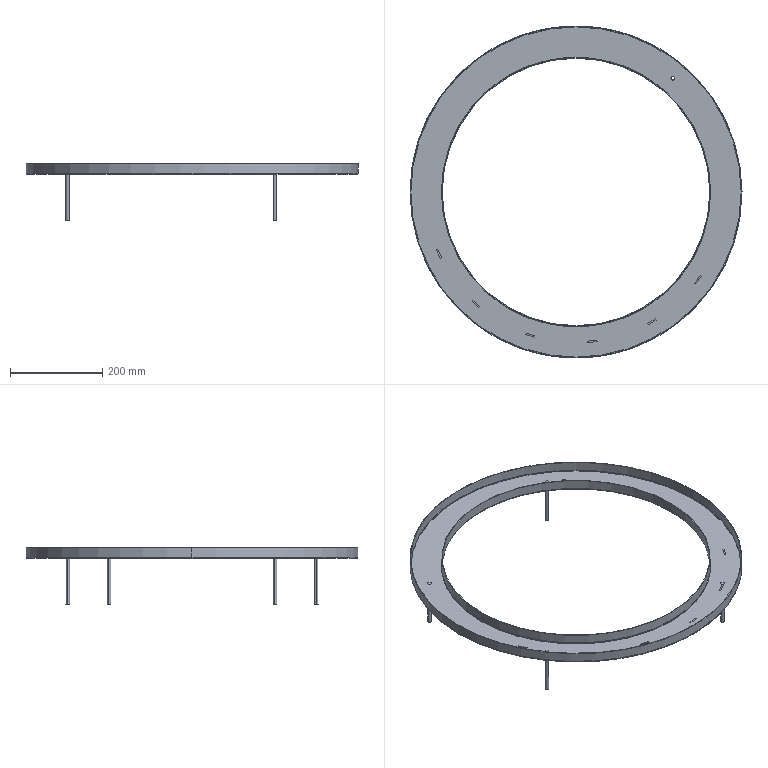Part | 1 solid | 64 faces | box 720 x 720 x 123 mm | volume 295569 mm3 | plane 38 | cylinder 18 | torus 8 | commonest cylinder face diameters 8 x10 580 x2 582.4 x2 717.6 x2 720 x2